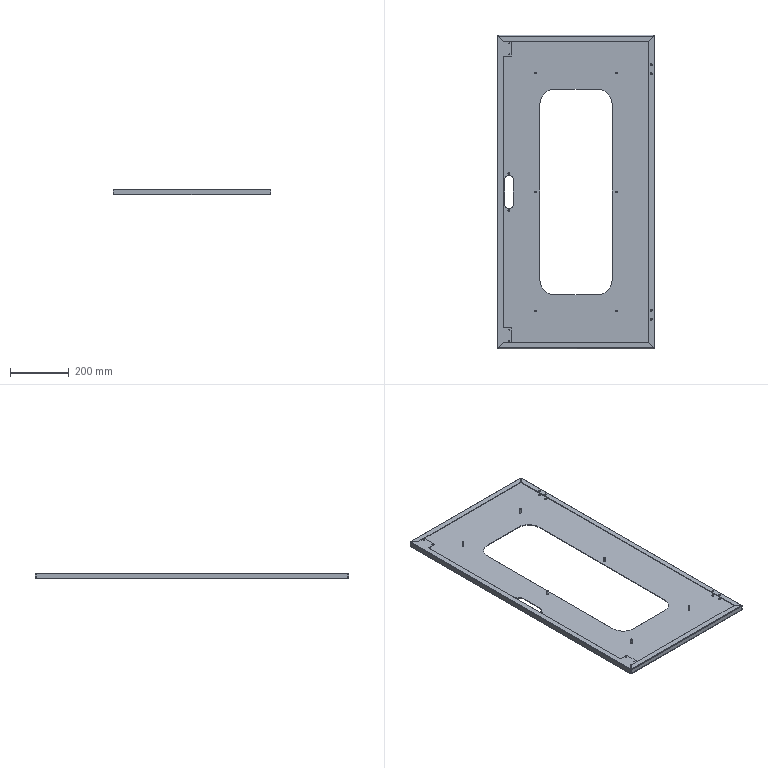Part | SolidWorks | features ICE 4, HoleWzd 3, EdgeFlange 2, Cut 1, FlatPattern 1, LPattern 1, SMBaseFlange 1, SheetMetal 1 | 1 solid | 134 faces | box 536 x 1066 x 20 mm | volume 1021642 mm3 | cylinder 62 | plane 56 | spline 16 | commonest cylinder face diameters 6.5 x16 5 x12 1.473 x8 3.3 x8 5.473 x8 7 x4